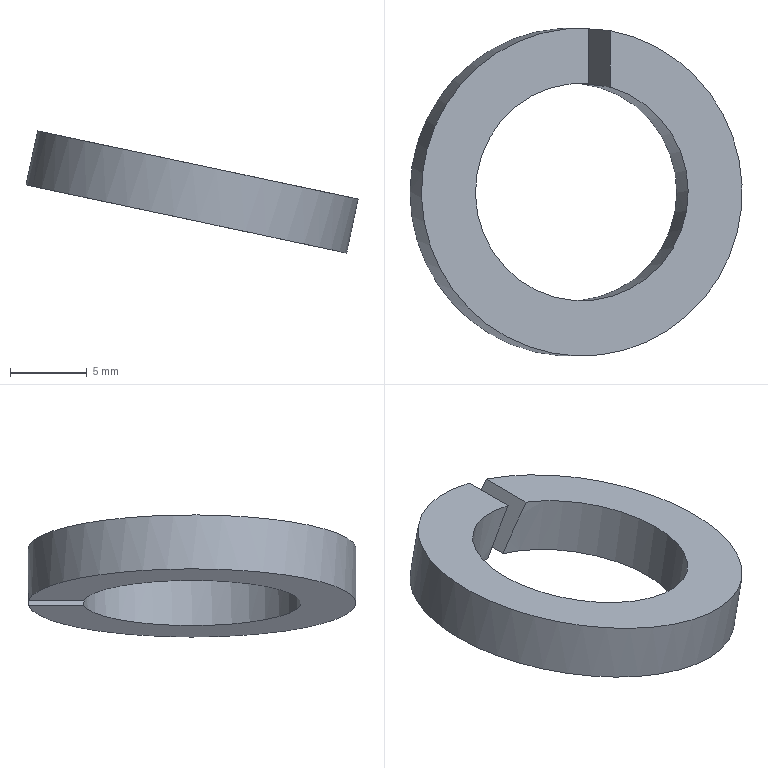Part | STEP file | 8902-14T spring washer | 1 solid | 6 faces | box 21.681 x 21.4 x 7.971 mm | volume 705.987 mm3 | plane 4 | cylinder 2 | commonest cylinder face diameters 14.2 x1 21.4 x1
STEP:
#1=CARTESIAN_POINT('',(0.,0.,0.));
#2=DIRECTION('',(0.,0.,1.));
#3=DIRECTION('',(1.,0.,0.));
#4=AXIS2_PLACEMENT_3D('',#1,#2,#3);
#5=CARTESIAN_POINT('',(2053.767,-218.824,-422.011));
#6=VERTEX_POINT('',#5);
#7=CARTESIAN_POINT('',(2053.767,-222.437,-422.011));
#8=VERTEX_POINT('',#7);
#9=CARTESIAN_POINT('',(2053.767,-229.5,-422.011));
#10=DIRECTION('',(0.,-1.,0.));
#11=VECTOR('',#10,1.);
#12=LINE('',#9,#11);
#13=CARTESIAN_POINT('',(2054.471,-229.5,-422.161));
#14=DIRECTION('',(-0.2079,0.,-0.9781));
#15=DIRECTION('',(0.,1.,0.));
#16=AXIS2_PLACEMENT_3D('',#13,#14,#15);
#17=PLANE('',#16);
#18=CARTESIAN_POINT('',(0.,-0.72));
#19=DIRECTION('',(-1.,0.));
#20=VECTOR('',#19,1.);
#21=LINE('',#18,#20);
#22=(GEOMETRIC_REPRESENTATION_CONTEXT(2)PARAMETRIC_REPRESENTATION_CONTEXT()REPRESENTATION_CONTEXT('',''));
#23=DEFINITIONAL_REPRESENTATION('',(#21),#22);
#24=PCURVE('',#17,#23);
#25=CARTESIAN_POINT('',(2055.66,-229.5,-418.733));
#26=DIRECTION('',(-0.866,0.,0.5));
#27=DIRECTION('',(0.,-1.,0.));
#28=AXIS2_PLACEMENT_3D('',#25,#26,#27);
#29=PLANE('',#28);
#30=CARTESIAN_POINT('',(0.,-3.785));
#31=DIRECTION('',(1.,0.));
#32=VECTOR('',#31,1.);
#33=LINE('',#30,#32);
#34=(GEOMETRIC_REPRESENTATION_CONTEXT(2)PARAMETRIC_REPRESENTATION_CONTEXT()REPRESENTATION_CONTEXT('',''));
#35=DEFINITIONAL_REPRESENTATION('',(#33),#34);
#36=PCURVE('',#29,#35);
#37=SURFACE_CURVE('',#12,(#24,#36),.PCURVE_S1.);
#38=EDGE_CURVE('',#6,#8,#37,.T.);
#39=ORIENTED_EDGE('',*,*,#38,.T.);
#40=CARTESIAN_POINT('',(2055.175,-222.437,-422.31));
#41=VERTEX_POINT('',#40);
#42=CARTESIAN_POINT('',(2054.471,-229.5,-422.161));
#43=DIRECTION('',(0.2079,0.,0.9781));
#44=DIRECTION('',(-0.9781,0.,0.2079));
#45=AXIS2_PLACEMENT_3D('',#42,#43,#44);
#46=CIRCLE('',#45,7.1);
#47=CARTESIAN_POINT('',(0.,-7.1));
#48=CARTESIAN_POINT('',(-12.298,-7.1));
#49=CARTESIAN_POINT('',(-6.149,3.55));
#50=CARTESIAN_POINT('',(0.,14.2));
#51=CARTESIAN_POINT('',(6.149,3.55));
#52=CARTESIAN_POINT('',(12.298,-7.1));
#53=CARTESIAN_POINT('',(0.,-7.1));
#54=(BOUNDED_CURVE()B_SPLINE_CURVE(2,(#47,#48,#49,#50,#51,#52,#53),.UNSPECIFIED.,.T.,.F.)B_SPLINE_CURVE_WITH_KNOTS((1,2,2,2,2,1),(-2.094,0.,2.094,4.189,6.283,8.378),.UNSPECIFIED.)CURVE()GEOMETRIC_REPRESENTATION_ITEM()RATIONAL_B_SPLINE_CURVE((1.,0.5,1.,0.5,1.,0.5,1.))REPRESENTATION_ITEM(''));
#55=(GEOMETRIC_REPRESENTATION_CONTEXT(2)PARAMETRIC_REPRESENTATION_CONTEXT()REPRESENTATION_CONTEXT('',''));
#56=DEFINITIONAL_REPRESENTATION('',(#54),#55);
#57=PCURVE('',#17,#56);
#58=CARTESIAN_POINT('',(2054.471,-229.5,-422.161));
#59=DIRECTION('',(0.2079,0.,0.9781));
#60=DIRECTION('',(-0.9781,0.,0.2079));
#61=AXIS2_PLACEMENT_3D('',#58,#59,#60);
#62=CYLINDRICAL_SURFACE('',#61,7.1);
#63=CARTESIAN_POINT('',(-6.283,0.));
#64=DIRECTION('',(1.,0.));
#65=VECTOR('',#64,1.);
#66=LINE('',#63,#65);
#67=(GEOMETRIC_REPRESENTATION_CONTEXT(2)PARAMETRIC_REPRESENTATION_CONTEXT()REPRESENTATION_CONTEXT('',''));
#68=DEFINITIONAL_REPRESENTATION('',(#66),#67);
#69=PCURVE('',#62,#68);
#70=SURFACE_CURVE('',#46,(#57,#69),.PCURVE_S1.);
#71=EDGE_CURVE('',#8,#41,#70,.T.);
#72=ORIENTED_EDGE('',*,*,#71,.T.);
#73=CARTESIAN_POINT('',(2055.175,-218.824,-422.31));
#74=VERTEX_POINT('',#73);
#75=CARTESIAN_POINT('',(2055.175,-229.5,-422.31));
#76=DIRECTION('',(0.,1.,0.));
#77=VECTOR('',#76,1.);
#78=LINE('',#75,#77);
#79=CARTESIAN_POINT('',(0.,0.72));
#80=DIRECTION('',(1.,0.));
#81=VECTOR('',#80,1.);
#82=LINE('',#79,#81);
#83=(GEOMETRIC_REPRESENTATION_CONTEXT(2)PARAMETRIC_REPRESENTATION_CONTEXT()REPRESENTATION_CONTEXT('',''));
#84=DEFINITIONAL_REPRESENTATION('',(#82),#83);
#85=PCURVE('',#17,#84);
#86=CARTESIAN_POINT('',(2055.175,-229.5,-422.31));
#87=DIRECTION('',(0.866,0.,-0.5));
#88=DIRECTION('',(0.,1.,0.));
#89=AXIS2_PLACEMENT_3D('',#86,#87,#88);
#90=PLANE('',#89);
#91=CARTESIAN_POINT('',(0.,0.));
#92=DIRECTION('',(1.,0.));
#93=VECTOR('',#92,1.);
#94=LINE('',#91,#93);
#95=(GEOMETRIC_REPRESENTATION_CONTEXT(2)PARAMETRIC_REPRESENTATION_CONTEXT()REPRESENTATION_CONTEXT('',''));
#96=DEFINITIONAL_REPRESENTATION('',(#94),#95);
#97=PCURVE('',#90,#96);
#98=SURFACE_CURVE('',#78,(#85,#97),.PCURVE_S1.);
#99=EDGE_CURVE('',#41,#74,#98,.T.);
#100=ORIENTED_EDGE('',*,*,#99,.T.);
#101=CARTESIAN_POINT('',(2054.471,-229.5,-422.161));
#102=DIRECTION('',(-0.2079,0.,-0.9781));
#103=DIRECTION('',(-0.9781,0.,0.2079));
#104=AXIS2_PLACEMENT_3D('',#101,#102,#103);
#105=CIRCLE('',#104,10.7);
#106=CARTESIAN_POINT('',(0.,0.));
#107=DIRECTION('',(0.,-1.));
#108=AXIS2_PLACEMENT_2D('',#106,#107);
#109=CIRCLE('',#108,10.7);
#110=(GEOMETRIC_REPRESENTATION_CONTEXT(2)PARAMETRIC_REPRESENTATION_CONTEXT()REPRESENTATION_CONTEXT('',''));
#111=DEFINITIONAL_REPRESENTATION('',(#109),#110);
#112=PCURVE('',#17,#111);
#113=CARTESIAN_POINT('',(2054.471,-229.5,-422.161));
#114=DIRECTION('',(0.2079,0.,0.9781));
#115=DIRECTION('',(-0.9781,0.,0.2079));
#116=AXIS2_PLACEMENT_3D('',#113,#114,#115);
#117=CYLINDRICAL_SURFACE('',#116,10.7);
#118=CARTESIAN_POINT('',(6.283,0.));
#119=DIRECTION('',(-1.,0.));
#120=VECTOR('',#119,1.);
#121=LINE('',#118,#120);
#122=(GEOMETRIC_REPRESENTATION_CONTEXT(2)PARAMETRIC_REPRESENTATION_CONTEXT()REPRESENTATION_CONTEXT('',''));
#123=DEFINITIONAL_REPRESENTATION('',(#121),#122);
#124=PCURVE('',#117,#123);
#125=SURFACE_CURVE('',#105,(#112,#124),.PCURVE_S1.);
#126=EDGE_CURVE('',#74,#6,#125,.T.);
#127=ORIENTED_EDGE('',*,*,#126,.T.);
#128=EDGE_LOOP('',(#39,#72,#100,#127));
#129=FACE_BOUND('',#128,.T.);
#130=ADVANCED_FACE('',(#129),#17,.T.);
#131=CARTESIAN_POINT('',(2055.66,-218.809,-418.733));
#132=VERTEX_POINT('',#131);
#133=CARTESIAN_POINT('',(2054.932,-229.5,-419.993));
#134=DIRECTION('',(-0.866,0.,0.5));
#135=DIRECTION('',(-0.5,0.,-0.866));
#136=AXIS2_PLACEMENT_3D('',#133,#134,#135);
#137=ELLIPSE('',#136,34.626,10.7);
#138=CARTESIAN_POINT('',(-1.613,3.6));
#139=CARTESIAN_POINT('',(-1.611,3.545));
#140=CARTESIAN_POINT('',(-1.608,3.436));
#141=CARTESIAN_POINT('',(-1.603,3.273));
#142=CARTESIAN_POINT('',(-1.598,3.109));
#143=CARTESIAN_POINT('',(-1.593,2.945));
#144=CARTESIAN_POINT('',(-1.588,2.782));
#145=CARTESIAN_POINT('',(-1.583,2.618));
#146=CARTESIAN_POINT('',(-1.578,2.454));
#147=CARTESIAN_POINT('',(-1.573,2.291));
#148=CARTESIAN_POINT('',(-1.568,2.127));
#149=CARTESIAN_POINT('',(-1.563,1.963));
#150=CARTESIAN_POINT('',(-1.558,1.799));
#151=CARTESIAN_POINT('',(-1.553,1.636));
#152=CARTESIAN_POINT('',(-1.548,1.472));
#153=CARTESIAN_POINT('',(-1.543,1.308));
#154=CARTESIAN_POINT('',(-1.538,1.145));
#155=CARTESIAN_POINT('',(-1.533,0.981));
#156=CARTESIAN_POINT('',(-1.528,0.8174));
#157=CARTESIAN_POINT('',(-1.523,0.6538));
#158=CARTESIAN_POINT('',(-1.518,0.4903));
#159=CARTESIAN_POINT('',(-1.513,0.3268));
#160=CARTESIAN_POINT('',(-1.508,0.1634));
#161=CARTESIAN_POINT('',(-1.505,0.05445));
#162=CARTESIAN_POINT('',(-1.503,0.));
#163=B_SPLINE_CURVE_WITH_KNOTS('',3,(#138,#139,#140,#141,#142,#143,#144,#145,#146,#147,#148,#149,#150,#151,#152,#153,#154,#155,#156,#157,#158,#159,#160,#161,#162),.UNSPECIFIED.,.F.,.F.,(4,1,1,1,1,1,1,1,1,1,1,1,1,1,1,1,1,1,1,1,1,1,4),(4.67,4.675,4.68,4.685,4.69,4.695,4.7,4.705,4.71,4.715,4.72,4.725,4.73,4.735,4.74,4.745,4.75,4.755,4.76,4.765,4.77,4.775,4.78),.QUASI_UNIFORM_KNOTS.);
#164=(GEOMETRIC_REPRESENTATION_CONTEXT(2)PARAMETRIC_REPRESENTATION_CONTEXT()REPRESENTATION_CONTEXT('',''));
#165=DEFINITIONAL_REPRESENTATION('',(#163),#164);
#166=PCURVE('',#117,#165);
#167=CARTESIAN_POINT('',(0.,-1.455));
#168=DIRECTION('',(0.,-1.));
#169=AXIS2_PLACEMENT_2D('',#167,#168);
#170=ELLIPSE('',#169,34.626,10.7);
#171=(GEOMETRIC_REPRESENTATION_CONTEXT(2)PARAMETRIC_REPRESENTATION_CONTEXT()REPRESENTATION_CONTEXT('',''));
#172=DEFINITIONAL_REPRESENTATION('',(#170),#171);
#173=PCURVE('',#29,#172);
#174=SURFACE_CURVE('',#137,(#166,#173),.PCURVE_S1.);
#175=EDGE_CURVE('',#132,#6,#174,.T.);
#176=ORIENTED_EDGE('',*,*,#175,.T.);
#177=ORIENTED_EDGE('',*,*,#126,.F.);
#178=CARTESIAN_POINT('',(2057.068,-218.968,-419.032));
#179=VERTEX_POINT('',#178);
#180=CARTESIAN_POINT('',(2054.011,-229.5,-424.328));
#181=DIRECTION('',(0.866,0.,-0.5));
#182=DIRECTION('',(-0.5,0.,-0.866));
#183=AXIS2_PLACEMENT_3D('',#180,#181,#182);
#184=ELLIPSE('',#183,34.626,10.7);
#185=CARTESIAN_POINT('',(4.645,0.));
#186=CARTESIAN_POINT('',(4.643,0.05486));
#187=CARTESIAN_POINT('',(4.64,0.1646));
#188=CARTESIAN_POINT('',(4.635,0.3291));
#189=CARTESIAN_POINT('',(4.63,0.4935));
#190=CARTESIAN_POINT('',(4.625,0.6578));
#191=CARTESIAN_POINT('',(4.62,0.8221));
#192=CARTESIAN_POINT('',(4.615,0.9863));
#193=CARTESIAN_POINT('',(4.61,1.15));
#194=CARTESIAN_POINT('',(4.605,1.315));
#195=CARTESIAN_POINT('',(4.6,1.478));
#196=CARTESIAN_POINT('',(4.595,1.642));
#197=CARTESIAN_POINT('',(4.59,1.806));
#198=CARTESIAN_POINT('',(4.585,1.97));
#199=CARTESIAN_POINT('',(4.58,2.133));
#200=CARTESIAN_POINT('',(4.575,2.297));
#201=CARTESIAN_POINT('',(4.57,2.46));
#202=CARTESIAN_POINT('',(4.565,2.623));
#203=CARTESIAN_POINT('',(4.56,2.786));
#204=CARTESIAN_POINT('',(4.555,2.949));
#205=CARTESIAN_POINT('',(4.55,3.112));
#206=CARTESIAN_POINT('',(4.545,3.275));
#207=CARTESIAN_POINT('',(4.54,3.438));
#208=CARTESIAN_POINT('',(4.537,3.546));
#209=CARTESIAN_POINT('',(4.535,3.6));
#210=B_SPLINE_CURVE_WITH_KNOTS('',3,(#185,#186,#187,#188,#189,#190,#191,#192,#193,#194,#195,#196,#197,#198,#199,#200,#201,#202,#203,#204,#205,#206,#207,#208,#209),.UNSPECIFIED.,.F.,.F.,(4,1,1,1,1,1,1,1,1,1,1,1,1,1,1,1,1,1,1,1,1,1,4),(1.638,1.643,1.648,1.653,1.658,1.663,1.668,1.673,1.678,1.683,1.688,1.693,1.698,1.703,1.708,1.713,1.718,1.723,1.728,1.733,1.738,1.743,1.748),.QUASI_UNIFORM_KNOTS.);
#211=(GEOMETRIC_REPRESENTATION_CONTEXT(2)PARAMETRIC_REPRESENTATION_CONTEXT()REPRESENTATION_CONTEXT('',''));
#212=DEFINITIONAL_REPRESENTATION('',(#210),#211);
#213=PCURVE('',#117,#212);
#214=CARTESIAN_POINT('',(0.,-2.33));
#215=DIRECTION('',(0.,-1.));
#216=AXIS2_PLACEMENT_2D('',#214,#215);
#217=ELLIPSE('',#216,34.626,10.7);
#218=(GEOMETRIC_REPRESENTATION_CONTEXT(2)PARAMETRIC_REPRESENTATION_CONTEXT()REPRESENTATION_CONTEXT('',''));
#219=DEFINITIONAL_REPRESENTATION('',(#217),#218);
#220=PCURVE('',#90,#219);
#221=SURFACE_CURVE('',#184,(#213,#220),.PCURVE_S1.);
#222=EDGE_CURVE('',#74,#179,#221,.T.);
#223=ORIENTED_EDGE('',*,*,#222,.T.);
#224=CARTESIAN_POINT('',(2055.22,-229.5,-418.639));
#225=DIRECTION('',(-0.2079,0.,-0.9781));
#226=DIRECTION('',(-0.9781,0.,0.2079));
#227=AXIS2_PLACEMENT_3D('',#224,#225,#226);
#228=CIRCLE('',#227,10.7);
#229=CARTESIAN_POINT('',(6.283,3.6));
#230=DIRECTION('',(-1.,0.));
#231=VECTOR('',#230,1.);
#232=LINE('',#229,#231);
#233=(GEOMETRIC_REPRESENTATION_CONTEXT(2)PARAMETRIC_REPRESENTATION_CONTEXT()REPRESENTATION_CONTEXT('',''));
#234=DEFINITIONAL_REPRESENTATION('',(#232),#233);
#235=PCURVE('',#117,#234);
#236=CARTESIAN_POINT('',(2055.22,-229.5,-418.639));
#237=DIRECTION('',(-0.2079,0.,-0.9781));
#238=DIRECTION('',(0.,1.,0.));
#239=AXIS2_PLACEMENT_3D('',#236,#237,#238);
#240=PLANE('',#239);
#241=CARTESIAN_POINT('',(0.,0.));
#242=DIRECTION('',(0.,-1.));
#243=AXIS2_PLACEMENT_2D('',#241,#242);
#244=CIRCLE('',#243,10.7);
#245=(GEOMETRIC_REPRESENTATION_CONTEXT(2)PARAMETRIC_REPRESENTATION_CONTEXT()REPRESENTATION_CONTEXT('',''));
#246=DEFINITIONAL_REPRESENTATION('',(#244),#245);
#247=PCURVE('',#240,#246);
#248=SURFACE_CURVE('',#228,(#235,#247),.PCURVE_S1.);
#249=EDGE_CURVE('',#179,#132,#248,.T.);
#250=ORIENTED_EDGE('',*,*,#249,.T.);
#251=EDGE_LOOP('',(#176,#177,#223,#250));
#252=FACE_BOUND('',#251,.T.);
#253=ADVANCED_FACE('',(#252),#117,.T.);
#254=ORIENTED_EDGE('',*,*,#71,.T.);
#255=CARTESIAN_POINT('',(2057.068,-222.656,-419.032));
#256=VERTEX_POINT('',#255);
#257=CARTESIAN_POINT('',(2054.011,-229.5,-424.328));
#258=DIRECTION('',(-0.866,0.,0.5));
#259=DIRECTION('',(-0.5,0.,-0.866));
#260=AXIS2_PLACEMENT_3D('',#257,#258,#259);
#261=ELLIPSE('',#260,22.976,7.1);
#262=CARTESIAN_POINT('',(4.443,3.6));
#263=CARTESIAN_POINT('',(4.446,3.546));
#264=CARTESIAN_POINT('',(4.451,3.439));
#265=CARTESIAN_POINT('',(4.458,3.278));
#266=CARTESIAN_POINT('',(4.466,3.117));
#267=CARTESIAN_POINT('',(4.473,2.955));
#268=CARTESIAN_POINT('',(4.481,2.793));
#269=CARTESIAN_POINT('',(4.489,2.63));
#270=CARTESIAN_POINT('',(4.496,2.468));
#271=CARTESIAN_POINT('',(4.504,2.305));
#272=CARTESIAN_POINT('',(4.512,2.141));
#273=CARTESIAN_POINT('',(4.519,1.978));
#274=CARTESIAN_POINT('',(4.527,1.814));
#275=CARTESIAN_POINT('',(4.535,1.65));
#276=CARTESIAN_POINT('',(4.542,1.486));
#277=CARTESIAN_POINT('',(4.55,1.322));
#278=CARTESIAN_POINT('',(4.557,1.157));
#279=CARTESIAN_POINT('',(4.565,0.9923));
#280=CARTESIAN_POINT('',(4.573,0.8274));
#281=CARTESIAN_POINT('',(4.58,0.6622));
#282=CARTESIAN_POINT('',(4.588,0.4969));
#283=CARTESIAN_POINT('',(4.596,0.3314));
#284=CARTESIAN_POINT('',(4.603,0.1658));
#285=CARTESIAN_POINT('',(4.608,0.05528));
#286=CARTESIAN_POINT('',(4.611,0.));
#287=B_SPLINE_CURVE_WITH_KNOTS('',3,(#262,#263,#264,#265,#266,#267,#268,#269,#270,#271,#272,#273,#274,#275,#276,#277,#278,#279,#280,#281,#282,#283,#284,#285,#286),.UNSPECIFIED.,.F.,.F.,(4,1,1,1,1,1,1,1,1,1,1,1,1,1,1,1,1,1,1,1,1,1,4),(4.443,4.451,4.458,4.466,4.473,4.481,4.489,4.496,4.504,4.512,4.519,4.527,4.535,4.542,4.55,4.557,4.565,4.573,4.58,4.588,4.596,4.603,4.611),.QUASI_UNIFORM_KNOTS.);
#288=(GEOMETRIC_REPRESENTATION_CONTEXT(2)PARAMETRIC_REPRESENTATION_CONTEXT()REPRESENTATION_CONTEXT('',''));
#289=DEFINITIONAL_REPRESENTATION('',(#287),#288);
#290=PCURVE('',#62,#289);
#291=CARTESIAN_POINT('',(0.,-25.306));
#292=CARTESIAN_POINT('',(-12.298,-25.306));
#293=CARTESIAN_POINT('',(-6.149,9.158));
#294=CARTESIAN_POINT('',(0.,43.622));
#295=CARTESIAN_POINT('',(6.149,9.158));
#296=CARTESIAN_POINT('',(12.298,-25.306));
#297=CARTESIAN_POINT('',(0.,-25.306));
#298=(BOUNDED_CURVE()B_SPLINE_CURVE(2,(#291,#292,#293,#294,#295,#296,#297),.UNSPECIFIED.,.T.,.F.)B_SPLINE_CURVE_WITH_KNOTS((1,2,2,2,2,1),(-2.094,0.,2.094,4.189,6.283,8.378),.UNSPECIFIED.)CURVE()GEOMETRIC_REPRESENTATION_ITEM()RATIONAL_B_SPLINE_CURVE((1.,0.5,1.,0.5,1.,0.5,1.))REPRESENTATION_ITEM(''));
#299=(GEOMETRIC_REPRESENTATION_CONTEXT(2)PARAMETRIC_REPRESENTATION_CONTEXT()REPRESENTATION_CONTEXT('',''));
#300=DEFINITIONAL_REPRESENTATION('',(#298),#299);
#301=PCURVE('',#90,#300);
#302=SURFACE_CURVE('',#261,(#290,#301),.PCURVE_S1.);
#303=EDGE_CURVE('',#256,#41,#302,.T.);
#304=ORIENTED_EDGE('',*,*,#303,.F.);
#305=CARTESIAN_POINT('',(2055.66,-222.414,-418.733));
#306=VERTEX_POINT('',#305);
#307=CARTESIAN_POINT('',(2055.22,-229.5,-418.639));
#308=DIRECTION('',(-0.2079,0.,-0.9781));
#309=DIRECTION('',(-0.9781,0.,0.2079));
#310=AXIS2_PLACEMENT_3D('',#307,#308,#309);
#311=CIRCLE('',#310,7.1);
#312=CARTESIAN_POINT('',(6.283,3.6));
#313=DIRECTION('',(-1.,0.));
#314=VECTOR('',#313,1.);
#315=LINE('',#312,#314);
#316=(GEOMETRIC_REPRESENTATION_CONTEXT(2)PARAMETRIC_REPRESENTATION_CONTEXT()REPRESENTATION_CONTEXT('',''));
#317=DEFINITIONAL_REPRESENTATION('',(#315),#316);
#318=PCURVE('',#62,#317);
#319=CARTESIAN_POINT('',(0.,0.));
#320=DIRECTION('',(0.,-1.));
#321=AXIS2_PLACEMENT_2D('',#319,#320);
#322=CIRCLE('',#321,7.1);
#323=(GEOMETRIC_REPRESENTATION_CONTEXT(2)PARAMETRIC_REPRESENTATION_CONTEXT()REPRESENTATION_CONTEXT('',''));
#324=DEFINITIONAL_REPRESENTATION('',(#322),#323);
#325=PCURVE('',#240,#324);
#326=SURFACE_CURVE('',#311,(#318,#325),.PCURVE_S1.);
#327=EDGE_CURVE('',#256,#306,#326,.T.);
#328=ORIENTED_EDGE('',*,*,#327,.T.);
#329=CARTESIAN_POINT('',(2054.932,-229.5,-419.993));
#330=DIRECTION('',(0.866,0.,-0.5));
#331=DIRECTION('',(-0.5,0.,-0.866));
#332=AXIS2_PLACEMENT_3D('',#329,#330,#331);
#333=ELLIPSE('',#332,22.976,7.1);
#334=CARTESIAN_POINT('',(-1.469,0.));
#335=CARTESIAN_POINT('',(-1.472,0.05434));
#336=CARTESIAN_POINT('',(-1.477,0.163));
#337=CARTESIAN_POINT('',(-1.484,0.3262));
#338=CARTESIAN_POINT('',(-1.492,0.4895));
#339=CARTESIAN_POINT('',(-1.499,0.6529));
#340=CARTESIAN_POINT('',(-1.507,0.8164));
#341=CARTESIAN_POINT('',(-1.514,0.9799));
#342=CARTESIAN_POINT('',(-1.522,1.144));
#343=CARTESIAN_POINT('',(-1.529,1.307));
#344=CARTESIAN_POINT('',(-1.537,1.471));
#345=CARTESIAN_POINT('',(-1.544,1.635));
#346=CARTESIAN_POINT('',(-1.552,1.799));
#347=CARTESIAN_POINT('',(-1.559,1.962));
#348=CARTESIAN_POINT('',(-1.567,2.126));
#349=CARTESIAN_POINT('',(-1.574,2.29));
#350=CARTESIAN_POINT('',(-1.582,2.454));
#351=CARTESIAN_POINT('',(-1.589,2.618));
#352=CARTESIAN_POINT('',(-1.597,2.782));
#353=CARTESIAN_POINT('',(-1.604,2.945));
#354=CARTESIAN_POINT('',(-1.612,3.109));
#355=CARTESIAN_POINT('',(-1.619,3.273));
#356=CARTESIAN_POINT('',(-1.627,3.436));
#357=CARTESIAN_POINT('',(-1.632,3.545));
#358=CARTESIAN_POINT('',(-1.634,3.6));
#359=B_SPLINE_CURVE_WITH_KNOTS('',3,(#334,#335,#336,#337,#338,#339,#340,#341,#342,#343,#344,#345,#346,#347,#348,#349,#350,#351,#352,#353,#354,#355,#356,#357,#358),.UNSPECIFIED.,.F.,.F.,(4,1,1,1,1,1,1,1,1,1,1,1,1,1,1,1,1,1,1,1,1,1,4),(1.469,1.477,1.484,1.492,1.499,1.507,1.514,1.522,1.529,1.537,1.544,1.552,1.559,1.567,1.574,1.582,1.589,1.597,1.604,1.612,1.619,1.627,1.634),.QUASI_UNIFORM_KNOTS.);
#360=(GEOMETRIC_REPRESENTATION_CONTEXT(2)PARAMETRIC_REPRESENTATION_CONTEXT()REPRESENTATION_CONTEXT('',''));
#361=DEFINITIONAL_REPRESENTATION('',(#359),#360);
#362=PCURVE('',#62,#361);
#363=CARTESIAN_POINT('',(0.,-24.431));
#364=CARTESIAN_POINT('',(-12.298,-24.431));
#365=CARTESIAN_POINT('',(-6.149,10.033));
#366=CARTESIAN_POINT('',(0.,44.497));
#367=CARTESIAN_POINT('',(6.149,10.033));
#368=CARTESIAN_POINT('',(12.298,-24.431));
#369=CARTESIAN_POINT('',(0.,-24.431));
#370=(BOUNDED_CURVE()B_SPLINE_CURVE(2,(#363,#364,#365,#366,#367,#368,#369),.UNSPECIFIED.,.T.,.F.)B_SPLINE_CURVE_WITH_KNOTS((1,2,2,2,2,1),(-2.094,0.,2.094,4.189,6.283,8.378),.UNSPECIFIED.)CURVE()GEOMETRIC_REPRESENTATION_ITEM()RATIONAL_B_SPLINE_CURVE((1.,0.5,1.,0.5,1.,0.5,1.))REPRESENTATION_ITEM(''));
#371=(GEOMETRIC_REPRESENTATION_CONTEXT(2)PARAMETRIC_REPRESENTATION_CONTEXT()REPRESENTATION_CONTEXT('',''));
#372=DEFINITIONAL_REPRESENTATION('',(#370),#371);
#373=PCURVE('',#29,#372);
#374=SURFACE_CURVE('',#333,(#362,#373),.PCURVE_S1.);
#375=EDGE_CURVE('',#8,#306,#374,.T.);
#376=ORIENTED_EDGE('',*,*,#375,.F.);
#377=EDGE_LOOP('',(#254,#304,#328,#376));
#378=FACE_BOUND('',#377,.F.);
#379=ADVANCED_FACE('',(#378),#62,.F.);
#380=CARTESIAN_POINT('',(2055.66,-229.5,-418.733));
#381=DIRECTION('',(0.,1.,0.));
#382=VECTOR('',#381,1.);
#383=LINE('',#380,#382);
#384=CARTESIAN_POINT('',(0.,0.4497));
#385=DIRECTION('',(1.,0.));
#386=VECTOR('',#385,1.);
#387=LINE('',#384,#386);
#388=(GEOMETRIC_REPRESENTATION_CONTEXT(2)PARAMETRIC_REPRESENTATION_CONTEXT()REPRESENTATION_CONTEXT('',''));
#389=DEFINITIONAL_REPRESENTATION('',(#387),#388);
#390=PCURVE('',#240,#389);
#391=CARTESIAN_POINT('',(0.,0.));
#392=DIRECTION('',(-1.,0.));
#393=VECTOR('',#392,1.);
#394=LINE('',#391,#393);
#395=(GEOMETRIC_REPRESENTATION_CONTEXT(2)PARAMETRIC_REPRESENTATION_CONTEXT()REPRESENTATION_CONTEXT('',''));
#396=DEFINITIONAL_REPRESENTATION('',(#394),#395);
#397=PCURVE('',#29,#396);
#398=SURFACE_CURVE('',#383,(#390,#397),.PCURVE_S1.);
#399=EDGE_CURVE('',#306,#132,#398,.T.);
#400=ORIENTED_EDGE('',*,*,#399,.T.);
#401=ORIENTED_EDGE('',*,*,#249,.F.);
#402=CARTESIAN_POINT('',(2057.068,-229.5,-419.032));
#403=DIRECTION('',(0.,-1.,0.));
#404=VECTOR('',#403,1.);
#405=LINE('',#402,#404);
#406=CARTESIAN_POINT('',(0.,1.89));
#407=DIRECTION('',(-1.,0.));
#408=VECTOR('',#407,1.);
#409=LINE('',#406,#408);
#410=(GEOMETRIC_REPRESENTATION_CONTEXT(2)PARAMETRIC_REPRESENTATION_CONTEXT()REPRESENTATION_CONTEXT('',''));
#411=DEFINITIONAL_REPRESENTATION('',(#409),#410);
#412=PCURVE('',#240,#411);
#413=CARTESIAN_POINT('',(0.,3.785));
#414=DIRECTION('',(-1.,0.));
#415=VECTOR('',#414,1.);
#416=LINE('',#413,#415);
#417=(GEOMETRIC_REPRESENTATION_CONTEXT(2)PARAMETRIC_REPRESENTATION_CONTEXT()REPRESENTATION_CONTEXT('',''));
#418=DEFINITIONAL_REPRESENTATION('',(#416),#417);
#419=PCURVE('',#90,#418);
#420=SURFACE_CURVE('',#405,(#412,#419),.PCURVE_S1.);
#421=EDGE_CURVE('',#179,#256,#420,.T.);
#422=ORIENTED_EDGE('',*,*,#421,.T.);
#423=ORIENTED_EDGE('',*,*,#327,.T.);
#424=EDGE_LOOP('',(#400,#401,#422,#423));
#425=FACE_BOUND('',#424,.T.);
#426=ADVANCED_FACE('',(#425),#240,.F.);
#427=ORIENTED_EDGE('',*,*,#375,.F.);
#428=ORIENTED_EDGE('',*,*,#38,.F.);
#429=ORIENTED_EDGE('',*,*,#175,.F.);
#430=ORIENTED_EDGE('',*,*,#399,.F.);
#431=EDGE_LOOP('',(#427,#428,#429,#430));
#432=FACE_BOUND('',#431,.T.);
#433=ADVANCED_FACE('',(#432),#29,.F.);
#434=ORIENTED_EDGE('',*,*,#303,.F.);
#435=ORIENTED_EDGE('',*,*,#421,.F.);
#436=ORIENTED_EDGE('',*,*,#222,.F.);
#437=ORIENTED_EDGE('',*,*,#99,.F.);
#438=EDGE_LOOP('',(#434,#435,#436,#437));
#439=FACE_BOUND('',#438,.T.);
#440=ADVANCED_FACE('',(#439),#90,.F.);
#441=CLOSED_SHELL('',(#130,#253,#379,#426,#433,#440));
#442=MANIFOLD_SOLID_BREP('',#441);
#443=(LENGTH_UNIT()NAMED_UNIT(*)SI_UNIT(.MILLI.,.METRE.));
#444=UNCERTAINTY_MEASURE_WITH_UNIT(LENGTH_MEASURE(0.0000001),#443,'','');
#445=(NAMED_UNIT(*)PLANE_ANGLE_UNIT()SI_UNIT($,.RADIAN.));
#446=(NAMED_UNIT(*)SI_UNIT($,.STERADIAN.)SOLID_ANGLE_UNIT());
#447=(GEOMETRIC_REPRESENTATION_CONTEXT(3)GLOBAL_UNCERTAINTY_ASSIGNED_CONTEXT((#444))GLOBAL_UNIT_ASSIGNED_CONTEXT((#443,#445,#446))REPRESENTATION_CONTEXT('',''));
#448=ADVANCED_BREP_SHAPE_REPRESENTATION('',(#4,#442),#447);